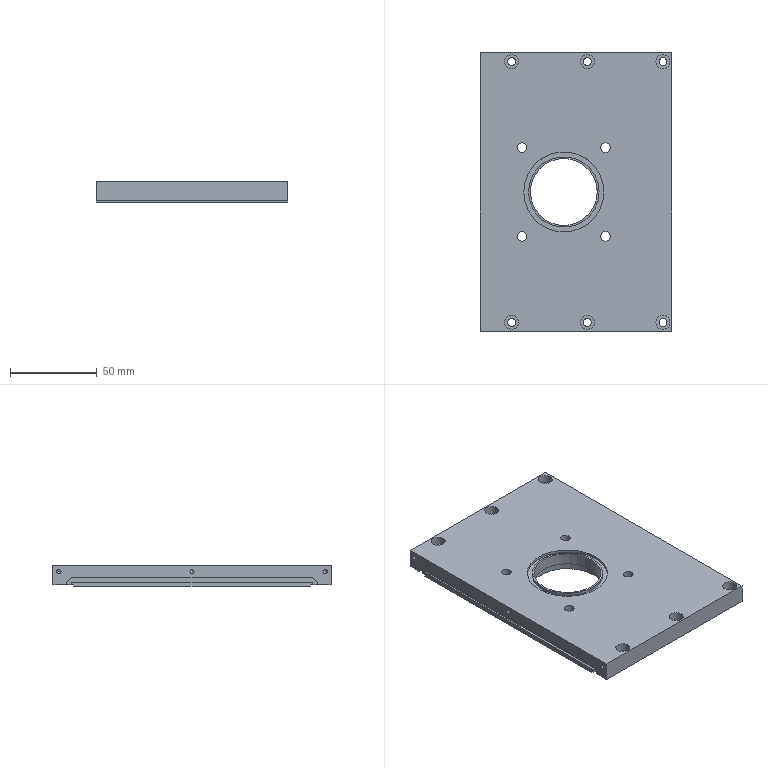NC program | NX | posted with a generic post | part box 110 x 160 x 12 mm
Whole program:
N10 G17 G21 G94 G90
(ZLEVEL_PROFILE_COPY_1 , TOOL : D2)
N12 T02 M6
N14 G54
N16 G17 G0 G90 X70.78 Y6.981 B0. C0. S9500 M3
N18 G43 Z30. H2
N20 Z0.156
N22 G94 G1 X70.776 Y6.978 Z0.11 F1100.
N24 X70.765 Y6.969 Z0.069
N26 X70.749 Y6.954 Z0.032
N28 X70.728 Y6.931 Z0.
N30 X70.703 Y6.9 Z-0.029
N32 X70.676 Y6.859 Z-0.054
N34 X70.648 Y6.81 Z-0.075
N36 X70.619 Y6.75 Z-0.093
N38 X70.591 Y6.679 Z-0.108
N40 X70.565 Y6.596 Z-0.12
N42 X70.542 Y6.501 Z-0.129
N44 X70.522 Y6.392 Z-0.136
N46 X70.508 Y6.27 Z-0.141
N48 X70.5 Y6.133 Z-0.144
N50 X70.499 Y5.981
N52 X70.503 Y5.811
N54 X70.5 Y4.5
N56 G2 X68.5 Y2.5 R2.
N58 G1 X-68.5
N60 G2 X-70.5 Y4.5 R2.
N62 G1 Y4.791
N64 X-70.497 Y5.981
N66 X-70.501 Y6.032
N68 X-70.514 Y6.075
N70 X-70.534 Y6.112
N72 X-70.56 Y6.142
N74 X-70.619 Y6.187
N76 X-70.701 Y6.221
N78 X-70.75 Y6.226
N80 X-70.799 Y6.221
N82 X-70.881 Y6.187
N84 X-70.94 Y6.142
N86 X-70.965 Y6.112
N88 X-70.985 Y6.075
N90 X-70.998 Y6.032
N92 X-71.003 Y5.981
N94 X-71. Y5.
N96 Y4.5
N98 G3 X-68.5 Y2. R2.5
N100 G1 X68.5
N102 G3 X71. Y4.5 R2.5
N104 G1 Y4.621
N106 Y5.981
N108 X70.996 Y6.033 Z-0.146
N110 X70.982 Y6.078 Z-0.149
N112 X70.962 Y6.115 Z-0.153
N114 X70.937 Y6.147 Z-0.159
N116 X70.878 Y6.193 Z-0.175
N118 X70.847 Y6.209 Z-0.184
N120 X70.796 Y6.228 Z-0.2
N122 X70.748 Y6.234 Z-0.217
N124 X70.699 Y6.228 Z-0.234
N126 X70.648 Y6.209 Z-0.25
N128 X70.588 Y6.173 Z-0.267
N130 X70.56 Y6.147 Z-0.274
N132 X70.535 Y6.115 Z-0.28
N134 X70.516 Y6.078 Z-0.285
N136 X70.503 Y6.033 Z-0.288
N138 X70.5 Y5.981 Z-0.289
N140 X70.503 Y5.811
N142 X70.5 Y4.5
N144 G2 X68.5 Y2.5 R2.
N146 G1 X-68.5
N148 G2 X-70.5 Y4.5 R2.
N150 G1 Y4.791
N152 X-70.497 Y5.981
N154 X-70.502 Y6.032
N156 X-70.515 Y6.075
N158 X-70.535 Y6.111
N160 X-70.56 Y6.142
N162 X-70.619 Y6.187
N164 X-70.701 Y6.22
N166 X-70.75 Y6.226
N168 X-70.799 Y6.22
N170 X-70.881 Y6.187
N172 X-70.94 Y6.142
N174 X-70.965 Y6.111
N176 X-70.985 Y6.075
N178 X-70.998 Y6.032
N180 X-71.003 Y5.981
N182 X-71. Y5.
N184 Y4.5
N186 G3 X-68.5 Y2. R2.5
N188 G1 X68.5
N190 G3 X71. Y4.5 R2.5
N192 G1 Y4.621
N194 Y5.981
N196 X70.995 Y6.033 Z-0.29
N198 X70.982 Y6.078 Z-0.293
N200 X70.962 Y6.115 Z-0.298
N202 X70.937 Y6.147 Z-0.304
N204 X70.878 Y6.193 Z-0.319
N206 X70.847 Y6.209 Z-0.328
N208 X70.796 Y6.227 Z-0.344
N210 X70.747 Y6.233 Z-0.361
N212 X70.699 Y6.227 Z-0.378
N214 X70.648 Y6.209 Z-0.394
N216 X70.588 Y6.172 Z-0.411
N218 X70.56 Y6.147 Z-0.418
N220 X70.535 Y6.115 Z-0.425
N222 X70.516 Y6.078 Z-0.429
N224 X70.504 Y6.033 Z-0.432
N226 X70.5 Y5.981 Z-0.433
N228 X70.503 Y5.811
N230 X70.5 Y4.5
N232 G2 X68.5 Y2.5 R2.
N234 G1 X-68.5
N236 G2 X-70.5 Y4.5 R2.
N238 G1 Y4.791
N240 X-70.497 Y5.981
N242 X-70.502 Y6.032
N244 X-70.515 Y6.075
N246 X-70.535 Y6.111
N248 X-70.56 Y6.142
N250 X-70.619 Y6.187
N252 X-70.701 Y6.22
N254 X-70.75 Y6.226
N256 X-70.799 Y6.22
N258 X-70.881 Y6.187
N260 X-70.94 Y6.142
N262 X-70.965 Y6.111
N264 X-70.985 Y6.075
N266 X-70.998 Y6.032
N268 X-71.003 Y5.981
N270 X-71. Y5.
N272 Y4.5
N274 G3 X-68.5 Y2. R2.5
N276 G1 X68.5
N278 G3 X71. Y4.5 R2.5
N280 G1 Y4.621
N282 Y5.981
N284 X70.995 Y6.033 Z-0.434
N286 X70.982 Y6.078 Z-0.437
N288 X70.962 Y6.115 Z-0.442
N290 X70.937 Y6.147 Z-0.448
N292 X70.877 Y6.193 Z-0.464
N294 X70.847 Y6.209 Z-0.472
N296 X70.796 Y6.227 Z-0.489
N298 X70.747 Y6.233 Z-0.506
N300 X70.699 Y6.227 Z-0.522
N302 X70.648 Y6.209 Z-0.539
N304 X70.588 Y6.172 Z-0.556
N306 X70.56 Y6.146 Z-0.563
N308 X70.535 Y6.115 Z-0.569
N310 X70.516 Y6.078 Z-0.574
N312 X70.504 Y6.033 Z-0.577
N314 X70.5 Y5.981 Z-0.578
N316 X70.504 Y5.811
N318 X70.5 Y4.5
N320 G2 X68.5 Y2.5 R2.
N322 G1 X-68.5
N324 G2 X-70.5 Y4.5 R2.
N326 G1 Y4.791
N328 X-70.498 Y5.981
N330 X-70.502 Y6.032
N332 X-70.515 Y6.075
N334 X-70.535 Y6.111
N336 X-70.56 Y6.142
N338 X-70.619 Y6.187
N340 X-70.701 Y6.22
N342 X-70.75 Y6.226
N344 X-70.799 Y6.22
N346 X-70.881 Y6.187
N348 X-70.94 Y6.142
N350 X-70.965 Y6.111
N352 X-70.985 Y6.075
N354 X-70.998 Y6.032
N356 X-71.002 Y5.981
N358 X-71. Y5.
N360 Y4.5
N362 G3 X-68.5 Y2. R2.5
N364 G1 X68.5
N366 G3 X71. Y4.5 R2.5
N368 G1 Y4.621
N370 X70.996 Y5.811
N372 X71. Y5.981
N374 X70.996 Y6.033 Z-0.579
N376 X70.984 Y6.077 Z-0.582
N378 X70.964 Y6.115 Z-0.587
N380 X70.939 Y6.146 Z-0.593
N382 X70.881 Y6.193 Z-0.608
N384 X70.85 Y6.209 Z-0.617
N386 X70.799 Y6.227 Z-0.633
N388 X70.75 Y6.233 Z-0.65
N390 X70.701 Y6.227 Z-0.667
N392 X70.65 Y6.209 Z-0.683
N394 X70.589 Y6.172 Z-0.7
N396 X70.561 Y6.146 Z-0.707
N398 X70.536 Y6.115 Z-0.713
N400 X70.517 Y6.077 Z-0.718
N402 X70.504 Y6.033 Z-0.721
N404 X70.5 Y5.981 Z-0.722
N406 X70.504 Y5.811
N408 X70.499 Y4.451
N410 G2 X68.5 Y2.5 R2.
N412 G1 X-68.5
N414 G2 X-70.5 Y4.5 R2.
N416 G1 Y4.791
N418 X-70.498 Y5.981
N420 X-70.502 Y6.031
N422 X-70.516 Y6.075
N424 X-70.535 Y6.111
N426 X-70.56 Y6.141
N428 X-70.619 Y6.186
N430 X-70.701 Y6.22
N432 X-70.75 Y6.225
N434 X-70.799 Y6.22
N436 X-70.881 Y6.186
N438 X-70.939 Y6.141
N440 X-70.964 Y6.111
N442 X-70.984 Y6.075
N444 X-70.997 Y6.031
N446 X-71.002 Y5.981
N448 X-71. Y5.
N450 Y4.5
N452 G3 X-68.5 Y2. R2.5
N454 G1 X68.5
N456 G3 X71. Y4.5 R2.5
N458 G1 Y4.621
N460 X70.996 Y5.811
N462 X70.999 Y5.981
N464 X70.996 Y6.033 Z-0.723
N466 X70.983 Y6.077 Z-0.726
N468 X70.964 Y6.115 Z-0.731
N470 X70.939 Y6.146 Z-0.737
N472 X70.881 Y6.192 Z-0.753
N474 X70.85 Y6.208 Z-0.761
N476 X70.799 Y6.227 Z-0.778
N478 X70.75 Y6.233 Z-0.794
N480 X70.701 Y6.227 Z-0.811
N482 X70.65 Y6.208 Z-0.828
N484 X70.589 Y6.172 Z-0.845
N486 X70.561 Y6.146 Z-0.852
N488 X70.536 Y6.115 Z-0.858
N490 X70.517 Y6.077 Z-0.863
N492 X70.504 Y6.033 Z-0.866
N494 X70.501 Y5.981 Z-0.867
N496 X70.505 Y5.811
N498 X70.499 Y4.451
N500 G2 X68.5 Y2.5 R2.
N502 G1 X-68.5
N504 G2 X-70.5 Y4.5 R2.
N506 G1 Y4.791
N508 X-70.498 Y5.981
N510 X-70.503 Y6.031
N512 X-70.516 Y6.074
N514 X-70.536 Y6.111
N516 X-70.561 Y6.141
N518 X-70.62 Y6.186
N520 X-70.701 Y6.219
N522 X-70.75 Y6.225
N524 X-70.799 Y6.219
N526 X-70.88 Y6.186
N528 X-70.939 Y6.141
N530 X-70.964 Y6.111
N532 X-70.984 Y6.074
N534 X-70.997 Y6.031
N536 X-71.002 Y5.981
N538 X-71. Y5.
N540 Y4.5
N542 G3 X-68.5 Y2. R2.5
N544 G1 X68.5
N546 G3 X71. Y4.5 R2.5
N548 G1 Y4.621
N550 X70.995 Y5.811
N552 X70.999 Y5.981
N554 X70.995 Y6.033 Z-0.868
N556 X70.983 Y6.077 Z-0.871
N558 X70.964 Y6.115 Z-0.875
N560 X70.939 Y6.146 Z-0.882
N562 X70.881 Y6.192 Z-0.897
N564 X70.85 Y6.208 Z-0.906
N566 X70.799 Y6.226 Z-0.922
N568 X70.75 Y6.232 Z-0.939
N570 X70.701 Y6.226 Z-0.956
N572 X70.65 Y6.208 Z-0.972
N574 X70.589 Y6.172 Z-0.989
N576 X70.561 Y6.146 Z-0.996
N578 X70.536 Y6.115 Z-1.002
N580 X70.517 Y6.077 Z-1.007
N582 X70.505 Y6.033 Z-1.01
N584 X70.501 Y5.981 Z-1.011
N586 X70.505 Y5.811
N588 X70.5 Y4.461
N590 G2 X68.5 Y2.5 R2.
N592 G1 X-68.5
N594 G2 X-70.5 Y4.5 R2.
N596 G1 Y4.791
N598 X-70.498 Y5.981
N600 X-70.503 Y6.031
N602 X-70.516 Y6.074
N604 X-70.536 Y6.111
N606 X-70.561 Y6.141
N608 X-70.62 Y6.186
N610 X-70.701 Y6.219
N612 X-70.75 Y6.225
N614 X-70.799 Y6.219
N616 X-70.88 Y6.186
N618 X-70.939 Y6.141
N620 X-70.964 Y6.111
N622 X-70.984 Y6.074
N624 X-70.997 Y6.031
N626 X-71.002 Y5.981
N628 X-71. Y5.
N630 Y4.5
N632 G3 X-68.5 Y2. R2.5
N634 G1 X68.5
N636 G3 X71. Y4.5 R2.5
N638 G1 Y4.621
N640 X70.995 Y5.811
N642 X70.999 Y5.981
N644 X70.995 Y6.033 Z-1.012
N646 X70.983 Y6.077 Z-1.015
N648 X70.964 Y6.115 Z-1.02
N650 X70.939 Y6.146 Z-1.026
N652 X70.88 Y6.192 Z-1.041
N654 X70.85 Y6.208 Z-1.05
N656 X70.799 Y6.226 Z-1.067
N658 X70.75 Y6.232 Z-1.083
N660 X70.701 Y6.226 Z-1.1
N662 X70.65 Y6.208 Z-1.116
N664 X70.589 Y6.171 Z-1.133
N666 X70.561 Y6.146 Z-1.141
N668 X70.536 Y6.115 Z-1.147
N670 X70.517 Y6.077 Z-1.151
N672 X70.505 Y6.033 Z-1.154
N674 X70.501 Y5.981 Z-1.156
N676 X70.505 Y5.811
N678 X70.5 Y4.5
N680 G2 X68.5 Y2.5 R2.
N682 G1 X-68.5
N684 G2 X-70.5 Y4.5 R2.
N686 G1 Y4.791
N688 X-70.499 Y5.981
N690 X-70.503 Y6.031
N692 X-70.516 Y6.074
N694 X-70.536 Y6.111
N696 X-70.561 Y6.141
N698 X-70.62 Y6.186
N700 X-70.701 Y6.219
N702 X-70.75 Y6.225
N704 X-70.799 Y6.219
N706 X-70.88 Y6.186
N708 X-70.939 Y6.141
N710 X-70.964 Y6.111
N712 X-70.984 Y6.074
N714 X-70.997 Y6.031
N716 X-71.001 Y5.981
N718 X-71. Y5.
N720 Y4.5
N722 G3 X-68.5 Y2. R2.5
N724 G1 X68.5
N726 G3 X71. Y4.535 R2.5
N728 G1 X70.994 Y5.811
N730 X70.999 Y5.981
N732 X70.995 Y6.033 Z-1.157
N734 X70.983 Y6.077 Z-1.16
N736 X70.964 Y6.114 Z-1.164
N738 X70.939 Y6.146 Z-1.17
N740 X70.88 Y6.192 Z-1.186
N742 X70.85 Y6.208 Z-1.195
N744 X70.799 Y6.226 Z-1.211
N746 X70.75 Y6.232 Z-1.228
N748 X70.701 Y6.226 Z-1.245
N750 X70.65 Y6.208 Z-1.261
N752 X70.589 Y6.171 Z-1.278
N754 X70.561 Y6.146 Z-1.285
N756 X70.537 Y6.114 Z-1.291
N758 X70.517 Y6.077 Z-1.296
N760 X70.505 Y6.033 Z-1.299
N762 X70.502 Y5.981 Z-1.3
N764 X70.506 Y5.811
N766 X70.5 Y4.5
N768 G2 X68.5 Y2.5 R2.
N770 G1 X-68.5
N772 G2 X-70.5 Y4.5 R2.
N774 G1 Y4.791
N776 X-70.499 Y5.981
N778 X-70.504 Y6.031
N780 X-70.517 Y6.074
N782 X-70.536 Y6.111
N784 X-70.561 Y6.141
N786 X-70.62 Y6.185
N788 X-70.701 Y6.219
N790 X-70.75 Y6.224
N792 X-70.799 Y6.219
N794 X-70.88 Y6.185
N796 X-70.939 Y6.141
N798 X-70.963 Y6.111
N800 X-70.983 Y6.074
N802 X-70.996 Y6.031
N804 X-71.001 Y5.981
N806 X-71. Y5.
N808 Y4.5
N810 G3 X-68.5 Y2. R2.5
N812 G1 X68.5
N814 G3 X71. Y4.535 R2.5
N816 G1 X70.994 Y5.811
N818 X70.998 Y5.981
N820 Y6.133 Z-1.299
N822 X70.991 Y6.27 Z-1.297
N824 X70.977 Y6.392 Z-1.292
N826 X70.959 Y6.501 Z-1.285
N828 X70.936 Y6.596 Z-1.276
N830 X70.91 Y6.679 Z-1.264
N832 X70.882 Y6.75 Z-1.249
N834 X70.854 Y6.81 Z-1.231
N836 X70.826 Y6.859 Z-1.209
N838 X70.799 Y6.899 Z-1.184
N840 X70.774 Y6.931 Z-1.156
N842 X70.754 Y6.954 Z-1.123
N844 X70.737 Y6.969 Z-1.087
N846 X70.727 Y6.978 Z-1.046
N848 X70.723 Y6.981 Z-1.
N850 G0 Z30.
N852 M5
(PLANAR_MILL_COPY_COPY_COPY_COPY_COPY_COPY_1_COPY_1_COPY_COPY , TOOL : D6A45)
N854 T01 M6
N856 G54
N858 G17 G0 G90 X-5.598 Y1.56 B0. C0. S9500 M3
N860 G43 Z30. H1
N862 Z0.84
N864 G94 G1 X0. Z-0.66 F1250.
N866 X68.5
N868 G3 X71.439 Y4.44 R2.94
N870 G1 X70.059
N872 G2 X68.5 Y2.94 R1.56
N874 G1 X-68.5
N876 G2 X-70.059 Y4.44 R1.56
N878 G1 X-71.439
N880 G3 X-68.5 Y1.56 R2.94
N882 G1 X0.
N884 G3 X0.866 Y2.06 R1.
N886 G1 Z0.84
N888 G0 Z30.
N890 M5
N892 M2